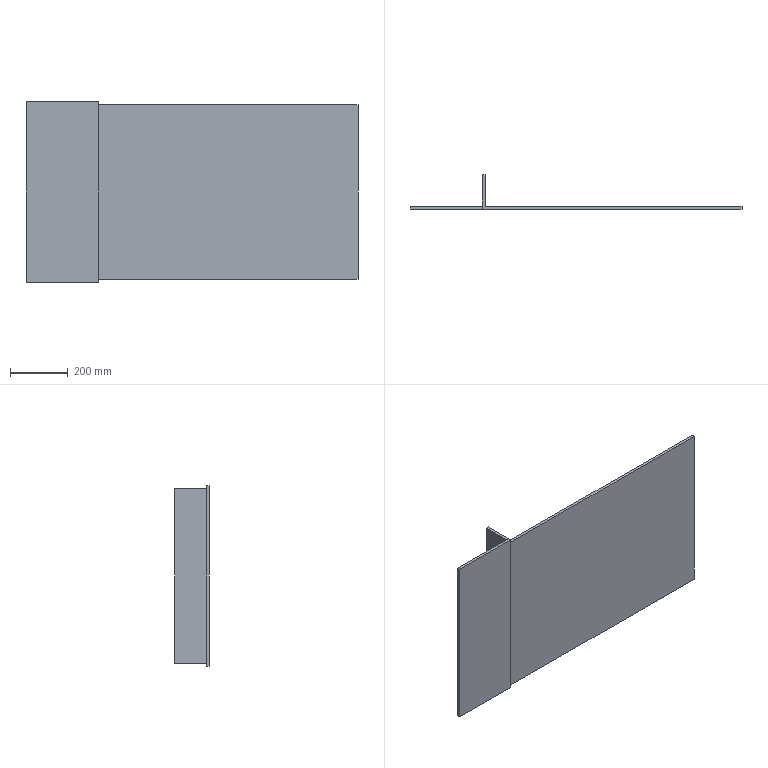Part | STEP file | zhihediban | 2 solids | 14 faces | box 1150 x 120 x 626 mm | volume 7685600 mm3 | plane 14
STEP:
#1=CARTESIAN_POINT('',(0.,0.,0.));
#2=DIRECTION('',(0.,0.,1.));
#3=DIRECTION('',(1.,0.,0.));
#4=AXIS2_PLACEMENT_3D('',#1,#2,#3);
#5=CARTESIAN_POINT('',(450.,5.,-303.));
#6=VERTEX_POINT('',#5);
#7=CARTESIAN_POINT('',(-440.,5.,-303.));
#8=VERTEX_POINT('',#7);
#9=CARTESIAN_POINT('',(-450.,5.,-303.));
#10=DIRECTION('',(-1.,0.,0.));
#11=VECTOR('',#10,1.);
#12=LINE('',#9,#11);
#13=CARTESIAN_POINT('',(0.,5.,0.));
#14=DIRECTION('',(0.,1.,0.));
#15=DIRECTION('',(0.,0.,1.));
#16=AXIS2_PLACEMENT_3D('',#13,#14,#15);
#17=PLANE('',#16);
#18=CARTESIAN_POINT('',(-303.,-450.));
#19=DIRECTION('',(0.,-1.));
#20=VECTOR('',#19,1.);
#21=LINE('',#18,#20);
#22=(GEOMETRIC_REPRESENTATION_CONTEXT(2)PARAMETRIC_REPRESENTATION_CONTEXT()REPRESENTATION_CONTEXT('',''));
#23=DEFINITIONAL_REPRESENTATION('',(#21),#22);
#24=PCURVE('',#17,#23);
#25=CARTESIAN_POINT('',(-450.,5.,-303.));
#26=DIRECTION('',(0.,0.,1.));
#27=DIRECTION('',(1.,0.,0.));
#28=AXIS2_PLACEMENT_3D('',#25,#26,#27);
#29=PLANE('',#28);
#30=CARTESIAN_POINT('',(0.,0.));
#31=DIRECTION('',(-1.,0.));
#32=VECTOR('',#31,1.);
#33=LINE('',#30,#32);
#34=(GEOMETRIC_REPRESENTATION_CONTEXT(2)PARAMETRIC_REPRESENTATION_CONTEXT()REPRESENTATION_CONTEXT('',''));
#35=DEFINITIONAL_REPRESENTATION('',(#33),#34);
#36=PCURVE('',#29,#35);
#37=SURFACE_CURVE('',#12,(#24,#36),.PCURVE_S1.);
#38=EDGE_CURVE('',#6,#8,#37,.T.);
#39=ORIENTED_EDGE('',*,*,#38,.T.);
#40=CARTESIAN_POINT('',(-440.,5.,303.));
#41=VERTEX_POINT('',#40);
#42=CARTESIAN_POINT('',(-440.,5.,-303.));
#43=DIRECTION('',(0.,0.,1.));
#44=VECTOR('',#43,1.);
#45=LINE('',#42,#44);
#46=CARTESIAN_POINT('',(-303.,-440.));
#47=DIRECTION('',(1.,0.));
#48=VECTOR('',#47,1.);
#49=LINE('',#46,#48);
#50=(GEOMETRIC_REPRESENTATION_CONTEXT(2)PARAMETRIC_REPRESENTATION_CONTEXT()REPRESENTATION_CONTEXT('',''));
#51=DEFINITIONAL_REPRESENTATION('',(#49),#50);
#52=PCURVE('',#17,#51);
#53=CARTESIAN_POINT('',(-440.,0.,0.));
#54=DIRECTION('',(1.,0.,0.));
#55=DIRECTION('',(0.,0.,-1.));
#56=AXIS2_PLACEMENT_3D('',#53,#54,#55);
#57=PLANE('',#56);
#58=CARTESIAN_POINT('',(303.,5.));
#59=DIRECTION('',(-1.,0.));
#60=VECTOR('',#59,1.);
#61=LINE('',#58,#60);
#62=(GEOMETRIC_REPRESENTATION_CONTEXT(2)PARAMETRIC_REPRESENTATION_CONTEXT()REPRESENTATION_CONTEXT('',''));
#63=DEFINITIONAL_REPRESENTATION('',(#61),#62);
#64=PCURVE('',#57,#63);
#65=SURFACE_CURVE('',#45,(#52,#64),.PCURVE_S1.);
#66=EDGE_CURVE('',#8,#41,#65,.T.);
#67=ORIENTED_EDGE('',*,*,#66,.T.);
#68=CARTESIAN_POINT('',(450.,5.,303.));
#69=VERTEX_POINT('',#68);
#70=CARTESIAN_POINT('',(-450.,5.,303.));
#71=DIRECTION('',(1.,0.,0.));
#72=VECTOR('',#71,1.);
#73=LINE('',#70,#72);
#74=CARTESIAN_POINT('',(303.,-450.));
#75=DIRECTION('',(0.,1.));
#76=VECTOR('',#75,1.);
#77=LINE('',#74,#76);
#78=(GEOMETRIC_REPRESENTATION_CONTEXT(2)PARAMETRIC_REPRESENTATION_CONTEXT()REPRESENTATION_CONTEXT('',''));
#79=DEFINITIONAL_REPRESENTATION('',(#77),#78);
#80=PCURVE('',#17,#79);
#81=CARTESIAN_POINT('',(-450.,5.,303.));
#82=DIRECTION('',(0.,0.,-1.));
#83=DIRECTION('',(-1.,0.,0.));
#84=AXIS2_PLACEMENT_3D('',#81,#82,#83);
#85=PLANE('',#84);
#86=CARTESIAN_POINT('',(0.,0.));
#87=DIRECTION('',(-1.,0.));
#88=VECTOR('',#87,1.);
#89=LINE('',#86,#88);
#90=(GEOMETRIC_REPRESENTATION_CONTEXT(2)PARAMETRIC_REPRESENTATION_CONTEXT()REPRESENTATION_CONTEXT('',''));
#91=DEFINITIONAL_REPRESENTATION('',(#89),#90);
#92=PCURVE('',#85,#91);
#93=SURFACE_CURVE('',#73,(#80,#92),.PCURVE_S1.);
#94=EDGE_CURVE('',#41,#69,#93,.T.);
#95=ORIENTED_EDGE('',*,*,#94,.T.);
#96=CARTESIAN_POINT('',(450.,5.,-303.));
#97=DIRECTION('',(0.,0.,-1.));
#98=VECTOR('',#97,1.);
#99=LINE('',#96,#98);
#100=CARTESIAN_POINT('',(-303.,450.));
#101=DIRECTION('',(-1.,0.));
#102=VECTOR('',#101,1.);
#103=LINE('',#100,#102);
#104=(GEOMETRIC_REPRESENTATION_CONTEXT(2)PARAMETRIC_REPRESENTATION_CONTEXT()REPRESENTATION_CONTEXT('',''));
#105=DEFINITIONAL_REPRESENTATION('',(#103),#104);
#106=PCURVE('',#17,#105);
#107=CARTESIAN_POINT('',(450.,5.,-303.));
#108=DIRECTION('',(-1.,0.,0.));
#109=DIRECTION('',(0.,0.,1.));
#110=AXIS2_PLACEMENT_3D('',#107,#108,#109);
#111=PLANE('',#110);
#112=CARTESIAN_POINT('',(0.,0.));
#113=DIRECTION('',(-1.,0.));
#114=VECTOR('',#113,1.);
#115=LINE('',#112,#114);
#116=(GEOMETRIC_REPRESENTATION_CONTEXT(2)PARAMETRIC_REPRESENTATION_CONTEXT()REPRESENTATION_CONTEXT('',''));
#117=DEFINITIONAL_REPRESENTATION('',(#115),#116);
#118=PCURVE('',#111,#117);
#119=SURFACE_CURVE('',#99,(#106,#118),.PCURVE_S1.);
#120=EDGE_CURVE('',#69,#6,#119,.T.);
#121=ORIENTED_EDGE('',*,*,#120,.T.);
#122=EDGE_LOOP('',(#39,#67,#95,#121));
#123=FACE_BOUND('',#122,.T.);
#124=ADVANCED_FACE('',(#123),#17,.T.);
#125=CARTESIAN_POINT('',(450.,-5.,303.));
#126=VERTEX_POINT('',#125);
#127=CARTESIAN_POINT('',(450.,-5.,-303.));
#128=VERTEX_POINT('',#127);
#129=CARTESIAN_POINT('',(450.,-5.,-303.));
#130=DIRECTION('',(0.,0.,-1.));
#131=VECTOR('',#130,1.);
#132=LINE('',#129,#131);
#133=CARTESIAN_POINT('',(0.,-10.));
#134=DIRECTION('',(-1.,0.));
#135=VECTOR('',#134,1.);
#136=LINE('',#133,#135);
#137=(GEOMETRIC_REPRESENTATION_CONTEXT(2)PARAMETRIC_REPRESENTATION_CONTEXT()REPRESENTATION_CONTEXT('',''));
#138=DEFINITIONAL_REPRESENTATION('',(#136),#137);
#139=PCURVE('',#111,#138);
#140=CARTESIAN_POINT('',(0.,-5.,0.));
#141=DIRECTION('',(0.,1.,0.));
#142=DIRECTION('',(0.,0.,1.));
#143=AXIS2_PLACEMENT_3D('',#140,#141,#142);
#144=PLANE('',#143);
#145=CARTESIAN_POINT('',(-303.,450.));
#146=DIRECTION('',(-1.,0.));
#147=VECTOR('',#146,1.);
#148=LINE('',#145,#147);
#149=(GEOMETRIC_REPRESENTATION_CONTEXT(2)PARAMETRIC_REPRESENTATION_CONTEXT()REPRESENTATION_CONTEXT('',''));
#150=DEFINITIONAL_REPRESENTATION('',(#148),#149);
#151=PCURVE('',#144,#150);
#152=SURFACE_CURVE('',#132,(#139,#151),.PCURVE_S1.);
#153=EDGE_CURVE('',#126,#128,#152,.T.);
#154=ORIENTED_EDGE('',*,*,#153,.T.);
#155=CARTESIAN_POINT('',(450.,5.,-303.));
#156=DIRECTION('',(0.,-1.,0.));
#157=VECTOR('',#156,1.);
#158=LINE('',#155,#157);
#159=CARTESIAN_POINT('',(0.,0.));
#160=DIRECTION('',(0.,-1.));
#161=VECTOR('',#160,1.);
#162=LINE('',#159,#161);
#163=(GEOMETRIC_REPRESENTATION_CONTEXT(2)PARAMETRIC_REPRESENTATION_CONTEXT()REPRESENTATION_CONTEXT('',''));
#164=DEFINITIONAL_REPRESENTATION('',(#162),#163);
#165=PCURVE('',#111,#164);
#166=CARTESIAN_POINT('',(900.,0.));
#167=DIRECTION('',(0.,-1.));
#168=VECTOR('',#167,1.);
#169=LINE('',#166,#168);
#170=(GEOMETRIC_REPRESENTATION_CONTEXT(2)PARAMETRIC_REPRESENTATION_CONTEXT()REPRESENTATION_CONTEXT('',''));
#171=DEFINITIONAL_REPRESENTATION('',(#169),#170);
#172=PCURVE('',#29,#171);
#173=SURFACE_CURVE('',#158,(#165,#172),.PCURVE_S1.);
#174=EDGE_CURVE('',#6,#128,#173,.T.);
#175=ORIENTED_EDGE('',*,*,#174,.F.);
#176=ORIENTED_EDGE('',*,*,#120,.F.);
#177=CARTESIAN_POINT('',(450.,5.,303.));
#178=DIRECTION('',(0.,-1.,0.));
#179=VECTOR('',#178,1.);
#180=LINE('',#177,#179);
#181=CARTESIAN_POINT('',(606.,0.));
#182=DIRECTION('',(0.,-1.));
#183=VECTOR('',#182,1.);
#184=LINE('',#181,#183);
#185=(GEOMETRIC_REPRESENTATION_CONTEXT(2)PARAMETRIC_REPRESENTATION_CONTEXT()REPRESENTATION_CONTEXT('',''));
#186=DEFINITIONAL_REPRESENTATION('',(#184),#185);
#187=PCURVE('',#111,#186);
#188=CARTESIAN_POINT('',(-900.,0.));
#189=DIRECTION('',(0.,-1.));
#190=VECTOR('',#189,1.);
#191=LINE('',#188,#190);
#192=(GEOMETRIC_REPRESENTATION_CONTEXT(2)PARAMETRIC_REPRESENTATION_CONTEXT()REPRESENTATION_CONTEXT('',''));
#193=DEFINITIONAL_REPRESENTATION('',(#191),#192);
#194=PCURVE('',#85,#193);
#195=SURFACE_CURVE('',#180,(#187,#194),.PCURVE_S1.);
#196=EDGE_CURVE('',#69,#126,#195,.T.);
#197=ORIENTED_EDGE('',*,*,#196,.T.);
#198=EDGE_LOOP('',(#154,#175,#176,#197));
#199=FACE_BOUND('',#198,.T.);
#200=ADVANCED_FACE('',(#199),#111,.F.);
#201=CARTESIAN_POINT('',(-450.,-5.,-303.));
#202=VERTEX_POINT('',#201);
#203=CARTESIAN_POINT('',(-450.,-5.,-303.));
#204=DIRECTION('',(-1.,0.,0.));
#205=VECTOR('',#204,1.);
#206=LINE('',#203,#205);
#207=CARTESIAN_POINT('',(0.,-10.));
#208=DIRECTION('',(-1.,0.));
#209=VECTOR('',#208,1.);
#210=LINE('',#207,#209);
#211=(GEOMETRIC_REPRESENTATION_CONTEXT(2)PARAMETRIC_REPRESENTATION_CONTEXT()REPRESENTATION_CONTEXT('',''));
#212=DEFINITIONAL_REPRESENTATION('',(#210),#211);
#213=PCURVE('',#29,#212);
#214=CARTESIAN_POINT('',(-303.,-450.));
#215=DIRECTION('',(0.,-1.));
#216=VECTOR('',#215,1.);
#217=LINE('',#214,#216);
#218=(GEOMETRIC_REPRESENTATION_CONTEXT(2)PARAMETRIC_REPRESENTATION_CONTEXT()REPRESENTATION_CONTEXT('',''));
#219=DEFINITIONAL_REPRESENTATION('',(#217),#218);
#220=PCURVE('',#144,#219);
#221=SURFACE_CURVE('',#206,(#213,#220),.PCURVE_S1.);
#222=EDGE_CURVE('',#128,#202,#221,.T.);
#223=ORIENTED_EDGE('',*,*,#222,.T.);
#224=CARTESIAN_POINT('',(-450.,115.,-303.));
#225=VERTEX_POINT('',#224);
#226=CARTESIAN_POINT('',(-450.,5.,-303.));
#227=DIRECTION('',(0.,-1.,0.));
#228=VECTOR('',#227,1.);
#229=LINE('',#226,#228);
#230=CARTESIAN_POINT('',(0.,0.));
#231=DIRECTION('',(0.,-1.));
#232=VECTOR('',#231,1.);
#233=LINE('',#230,#232);
#234=(GEOMETRIC_REPRESENTATION_CONTEXT(2)PARAMETRIC_REPRESENTATION_CONTEXT()REPRESENTATION_CONTEXT('',''));
#235=DEFINITIONAL_REPRESENTATION('',(#233),#234);
#236=PCURVE('',#29,#235);
#237=CARTESIAN_POINT('',(-450.,5.,-303.));
#238=DIRECTION('',(1.,0.,0.));
#239=DIRECTION('',(0.,0.,-1.));
#240=AXIS2_PLACEMENT_3D('',#237,#238,#239);
#241=PLANE('',#240);
#242=CARTESIAN_POINT('',(0.,0.));
#243=DIRECTION('',(0.,-1.));
#244=VECTOR('',#243,1.);
#245=LINE('',#242,#244);
#246=(GEOMETRIC_REPRESENTATION_CONTEXT(2)PARAMETRIC_REPRESENTATION_CONTEXT()REPRESENTATION_CONTEXT('',''));
#247=DEFINITIONAL_REPRESENTATION('',(#245),#246);
#248=PCURVE('',#241,#247);
#249=SURFACE_CURVE('',#229,(#236,#248),.PCURVE_S1.);
#250=EDGE_CURVE('',#225,#202,#249,.T.);
#251=ORIENTED_EDGE('',*,*,#250,.F.);
#252=CARTESIAN_POINT('',(-440.,115.,-303.));
#253=VERTEX_POINT('',#252);
#254=CARTESIAN_POINT('',(-440.,115.,-303.));
#255=DIRECTION('',(-1.,0.,0.));
#256=VECTOR('',#255,1.);
#257=LINE('',#254,#256);
#258=CARTESIAN_POINT('',(10.,110.));
#259=DIRECTION('',(-1.,0.));
#260=VECTOR('',#259,1.);
#261=LINE('',#258,#260);
#262=(GEOMETRIC_REPRESENTATION_CONTEXT(2)PARAMETRIC_REPRESENTATION_CONTEXT()REPRESENTATION_CONTEXT('',''));
#263=DEFINITIONAL_REPRESENTATION('',(#261),#262);
#264=PCURVE('',#29,#263);
#265=CARTESIAN_POINT('',(-440.,115.,-303.));
#266=DIRECTION('',(0.,1.,0.));
#267=DIRECTION('',(0.,0.,1.));
#268=AXIS2_PLACEMENT_3D('',#265,#266,#267);
#269=PLANE('',#268);
#270=CARTESIAN_POINT('',(0.,0.));
#271=DIRECTION('',(0.,-1.));
#272=VECTOR('',#271,1.);
#273=LINE('',#270,#272);
#274=(GEOMETRIC_REPRESENTATION_CONTEXT(2)PARAMETRIC_REPRESENTATION_CONTEXT()REPRESENTATION_CONTEXT('',''));
#275=DEFINITIONAL_REPRESENTATION('',(#273),#274);
#276=PCURVE('',#269,#275);
#277=SURFACE_CURVE('',#257,(#264,#276),.PCURVE_S1.);
#278=EDGE_CURVE('',#253,#225,#277,.T.);
#279=ORIENTED_EDGE('',*,*,#278,.F.);
#280=CARTESIAN_POINT('',(-440.,5.,-303.));
#281=DIRECTION('',(0.,-1.,0.));
#282=VECTOR('',#281,1.);
#283=LINE('',#280,#282);
#284=CARTESIAN_POINT('',(10.,0.));
#285=DIRECTION('',(0.,-1.));
#286=VECTOR('',#285,1.);
#287=LINE('',#284,#286);
#288=(GEOMETRIC_REPRESENTATION_CONTEXT(2)PARAMETRIC_REPRESENTATION_CONTEXT()REPRESENTATION_CONTEXT('',''));
#289=DEFINITIONAL_REPRESENTATION('',(#287),#288);
#290=PCURVE('',#29,#289);
#291=CARTESIAN_POINT('',(303.,5.));
#292=DIRECTION('',(0.,-1.));
#293=VECTOR('',#292,1.);
#294=LINE('',#291,#293);
#295=(GEOMETRIC_REPRESENTATION_CONTEXT(2)PARAMETRIC_REPRESENTATION_CONTEXT()REPRESENTATION_CONTEXT('',''));
#296=DEFINITIONAL_REPRESENTATION('',(#294),#295);
#297=PCURVE('',#57,#296);
#298=SURFACE_CURVE('',#283,(#290,#297),.PCURVE_S1.);
#299=EDGE_CURVE('',#253,#8,#298,.T.);
#300=ORIENTED_EDGE('',*,*,#299,.T.);
#301=ORIENTED_EDGE('',*,*,#38,.F.);
#302=ORIENTED_EDGE('',*,*,#174,.T.);
#303=EDGE_LOOP('',(#223,#251,#279,#300,#301,#302));
#304=FACE_BOUND('',#303,.T.);
#305=ADVANCED_FACE('',(#304),#29,.F.);
#306=CARTESIAN_POINT('',(-450.,-5.,303.));
#307=VERTEX_POINT('',#306);
#308=CARTESIAN_POINT('',(-450.,-5.,-303.));
#309=DIRECTION('',(0.,0.,1.));
#310=VECTOR('',#309,1.);
#311=LINE('',#308,#310);
#312=CARTESIAN_POINT('',(0.,-10.));
#313=DIRECTION('',(-1.,0.));
#314=VECTOR('',#313,1.);
#315=LINE('',#312,#314);
#316=(GEOMETRIC_REPRESENTATION_CONTEXT(2)PARAMETRIC_REPRESENTATION_CONTEXT()REPRESENTATION_CONTEXT('',''));
#317=DEFINITIONAL_REPRESENTATION('',(#315),#316);
#318=PCURVE('',#241,#317);
#319=CARTESIAN_POINT('',(-303.,-450.));
#320=DIRECTION('',(1.,0.));
#321=VECTOR('',#320,1.);
#322=LINE('',#319,#321);
#323=(GEOMETRIC_REPRESENTATION_CONTEXT(2)PARAMETRIC_REPRESENTATION_CONTEXT()REPRESENTATION_CONTEXT('',''));
#324=DEFINITIONAL_REPRESENTATION('',(#322),#323);
#325=PCURVE('',#144,#324);
#326=SURFACE_CURVE('',#311,(#318,#325),.PCURVE_S1.);
#327=EDGE_CURVE('',#202,#307,#326,.T.);
#328=ORIENTED_EDGE('',*,*,#327,.T.);
#329=CARTESIAN_POINT('',(-450.,115.,303.));
#330=VERTEX_POINT('',#329);
#331=CARTESIAN_POINT('',(-450.,5.,303.));
#332=DIRECTION('',(0.,-1.,0.));
#333=VECTOR('',#332,1.);
#334=LINE('',#331,#333);
#335=CARTESIAN_POINT('',(-606.,0.));
#336=DIRECTION('',(0.,-1.));
#337=VECTOR('',#336,1.);
#338=LINE('',#335,#337);
#339=(GEOMETRIC_REPRESENTATION_CONTEXT(2)PARAMETRIC_REPRESENTATION_CONTEXT()REPRESENTATION_CONTEXT('',''));
#340=DEFINITIONAL_REPRESENTATION('',(#338),#339);
#341=PCURVE('',#241,#340);
#342=CARTESIAN_POINT('',(0.,0.));
#343=DIRECTION('',(0.,-1.));
#344=VECTOR('',#343,1.);
#345=LINE('',#342,#344);
#346=(GEOMETRIC_REPRESENTATION_CONTEXT(2)PARAMETRIC_REPRESENTATION_CONTEXT()REPRESENTATION_CONTEXT('',''));
#347=DEFINITIONAL_REPRESENTATION('',(#345),#346);
#348=PCURVE('',#85,#347);
#349=SURFACE_CURVE('',#334,(#341,#348),.PCURVE_S1.);
#350=EDGE_CURVE('',#330,#307,#349,.T.);
#351=ORIENTED_EDGE('',*,*,#350,.F.);
#352=CARTESIAN_POINT('',(-450.,115.,-303.));
#353=DIRECTION('',(0.,0.,-1.));
#354=VECTOR('',#353,1.);
#355=LINE('',#352,#354);
#356=CARTESIAN_POINT('',(0.,110.));
#357=DIRECTION('',(1.,0.));
#358=VECTOR('',#357,1.);
#359=LINE('',#356,#358);
#360=(GEOMETRIC_REPRESENTATION_CONTEXT(2)PARAMETRIC_REPRESENTATION_CONTEXT()REPRESENTATION_CONTEXT('',''));
#361=DEFINITIONAL_REPRESENTATION('',(#359),#360);
#362=PCURVE('',#241,#361);
#363=CARTESIAN_POINT('',(0.,-10.));
#364=DIRECTION('',(-1.,0.));
#365=VECTOR('',#364,1.);
#366=LINE('',#363,#365);
#367=(GEOMETRIC_REPRESENTATION_CONTEXT(2)PARAMETRIC_REPRESENTATION_CONTEXT()REPRESENTATION_CONTEXT('',''));
#368=DEFINITIONAL_REPRESENTATION('',(#366),#367);
#369=PCURVE('',#269,#368);
#370=SURFACE_CURVE('',#355,(#362,#369),.PCURVE_S1.);
#371=EDGE_CURVE('',#330,#225,#370,.T.);
#372=ORIENTED_EDGE('',*,*,#371,.T.);
#373=ORIENTED_EDGE('',*,*,#250,.T.);
#374=EDGE_LOOP('',(#328,#351,#372,#373));
#375=FACE_BOUND('',#374,.T.);
#376=ADVANCED_FACE('',(#375),#241,.F.);
#377=CARTESIAN_POINT('',(-450.,-5.,303.));
#378=DIRECTION('',(1.,0.,0.));
#379=VECTOR('',#378,1.);
#380=LINE('',#377,#379);
#381=CARTESIAN_POINT('',(0.,-10.));
#382=DIRECTION('',(-1.,0.));
#383=VECTOR('',#382,1.);
#384=LINE('',#381,#383);
#385=(GEOMETRIC_REPRESENTATION_CONTEXT(2)PARAMETRIC_REPRESENTATION_CONTEXT()REPRESENTATION_CONTEXT('',''));
#386=DEFINITIONAL_REPRESENTATION('',(#384),#385);
#387=PCURVE('',#85,#386);
#388=CARTESIAN_POINT('',(303.,-450.));
#389=DIRECTION('',(0.,1.));
#390=VECTOR('',#389,1.);
#391=LINE('',#388,#390);
#392=(GEOMETRIC_REPRESENTATION_CONTEXT(2)PARAMETRIC_REPRESENTATION_CONTEXT()REPRESENTATION_CONTEXT('',''));
#393=DEFINITIONAL_REPRESENTATION('',(#391),#392);
#394=PCURVE('',#144,#393);
#395=SURFACE_CURVE('',#380,(#387,#394),.PCURVE_S1.);
#396=EDGE_CURVE('',#307,#126,#395,.T.);
#397=ORIENTED_EDGE('',*,*,#396,.T.);
#398=ORIENTED_EDGE('',*,*,#196,.F.);
#399=ORIENTED_EDGE('',*,*,#94,.F.);
#400=CARTESIAN_POINT('',(-440.,115.,303.));
#401=VERTEX_POINT('',#400);
#402=CARTESIAN_POINT('',(-440.,5.,303.));
#403=DIRECTION('',(0.,1.,0.));
#404=VECTOR('',#403,1.);
#405=LINE('',#402,#404);
#406=CARTESIAN_POINT('',(-10.,0.));
#407=DIRECTION('',(0.,1.));
#408=VECTOR('',#407,1.);
#409=LINE('',#406,#408);
#410=(GEOMETRIC_REPRESENTATION_CONTEXT(2)PARAMETRIC_REPRESENTATION_CONTEXT()REPRESENTATION_CONTEXT('',''));
#411=DEFINITIONAL_REPRESENTATION('',(#409),#410);
#412=PCURVE('',#85,#411);
#413=CARTESIAN_POINT('',(-303.,5.));
#414=DIRECTION('',(0.,1.));
#415=VECTOR('',#414,1.);
#416=LINE('',#413,#415);
#417=(GEOMETRIC_REPRESENTATION_CONTEXT(2)PARAMETRIC_REPRESENTATION_CONTEXT()REPRESENTATION_CONTEXT('',''));
#418=DEFINITIONAL_REPRESENTATION('',(#416),#417);
#419=PCURVE('',#57,#418);
#420=SURFACE_CURVE('',#405,(#412,#419),.PCURVE_S1.);
#421=EDGE_CURVE('',#41,#401,#420,.T.);
#422=ORIENTED_EDGE('',*,*,#421,.T.);
#423=CARTESIAN_POINT('',(-440.,115.,303.));
#424=DIRECTION('',(-1.,0.,0.));
#425=VECTOR('',#424,1.);
#426=LINE('',#423,#425);
#427=CARTESIAN_POINT('',(-10.,110.));
#428=DIRECTION('',(1.,0.));
#429=VECTOR('',#428,1.);
#430=LINE('',#427,#429);
#431=(GEOMETRIC_REPRESENTATION_CONTEXT(2)PARAMETRIC_REPRESENTATION_CONTEXT()REPRESENTATION_CONTEXT('',''));
#432=DEFINITIONAL_REPRESENTATION('',(#430),#431);
#433=PCURVE('',#85,#432);
#434=CARTESIAN_POINT('',(606.,0.));
#435=DIRECTION('',(0.,-1.));
#436=VECTOR('',#435,1.);
#437=LINE('',#434,#436);
#438=(GEOMETRIC_REPRESENTATION_CONTEXT(2)PARAMETRIC_REPRESENTATION_CONTEXT()REPRESENTATION_CONTEXT('',''));
#439=DEFINITIONAL_REPRESENTATION('',(#437),#438);
#440=PCURVE('',#269,#439);
#441=SURFACE_CURVE('',#426,(#433,#440),.PCURVE_S1.);
#442=EDGE_CURVE('',#401,#330,#441,.T.);
#443=ORIENTED_EDGE('',*,*,#442,.T.);
#444=ORIENTED_EDGE('',*,*,#350,.T.);
#445=EDGE_LOOP('',(#397,#398,#399,#422,#443,#444));
#446=FACE_BOUND('',#445,.T.);
#447=ADVANCED_FACE('',(#446),#85,.F.);
#448=ORIENTED_EDGE('',*,*,#153,.F.);
#449=ORIENTED_EDGE('',*,*,#396,.F.);
#450=ORIENTED_EDGE('',*,*,#327,.F.);
#451=ORIENTED_EDGE('',*,*,#222,.F.);
#452=EDGE_LOOP('',(#448,#449,#450,#451));
#453=FACE_BOUND('',#452,.T.);
#454=ADVANCED_FACE('',(#453),#144,.F.);
#455=ORIENTED_EDGE('',*,*,#371,.F.);
#456=ORIENTED_EDGE('',*,*,#442,.F.);
#457=CARTESIAN_POINT('',(-440.,115.,-303.));
#458=DIRECTION('',(0.,0.,-1.));
#459=VECTOR('',#458,1.);
#460=LINE('',#457,#459);
#461=CARTESIAN_POINT('',(0.,0.));
#462=DIRECTION('',(-1.,0.));
#463=VECTOR('',#462,1.);
#464=LINE('',#461,#463);
#465=(GEOMETRIC_REPRESENTATION_CONTEXT(2)PARAMETRIC_REPRESENTATION_CONTEXT()REPRESENTATION_CONTEXT('',''));
#466=DEFINITIONAL_REPRESENTATION('',(#464),#465);
#467=PCURVE('',#269,#466);
#468=CARTESIAN_POINT('',(303.,115.));
#469=DIRECTION('',(1.,0.));
#470=VECTOR('',#469,1.);
#471=LINE('',#468,#470);
#472=(GEOMETRIC_REPRESENTATION_CONTEXT(2)PARAMETRIC_REPRESENTATION_CONTEXT()REPRESENTATION_CONTEXT('',''));
#473=DEFINITIONAL_REPRESENTATION('',(#471),#472);
#474=PCURVE('',#57,#473);
#475=SURFACE_CURVE('',#460,(#467,#474),.PCURVE_S1.);
#476=EDGE_CURVE('',#401,#253,#475,.T.);
#477=ORIENTED_EDGE('',*,*,#476,.T.);
#478=ORIENTED_EDGE('',*,*,#278,.T.);
#479=EDGE_LOOP('',(#455,#456,#477,#478));
#480=FACE_BOUND('',#479,.T.);
#481=ADVANCED_FACE('',(#480),#269,.T.);
#482=ORIENTED_EDGE('',*,*,#299,.F.);
#483=ORIENTED_EDGE('',*,*,#476,.F.);
#484=ORIENTED_EDGE('',*,*,#421,.F.);
#485=ORIENTED_EDGE('',*,*,#66,.F.);
#486=EDGE_LOOP('',(#482,#483,#484,#485));
#487=FACE_BOUND('',#486,.T.);
#488=ADVANCED_FACE('',(#487),#57,.T.);
#489=CLOSED_SHELL('',(#124,#200,#305,#376,#447,#454,#481,#488));
#490=MANIFOLD_SOLID_BREP('',#489);
#491=CARTESIAN_POINT('',(-700.,5.,313.));
#492=VERTEX_POINT('',#491);
#493=CARTESIAN_POINT('',(-700.,5.,-313.));
#494=VERTEX_POINT('',#493);
#495=CARTESIAN_POINT('',(-700.,5.,313.));
#496=DIRECTION('',(0.,0.,-1.));
#497=VECTOR('',#496,1.);
#498=LINE('',#495,#497);
#499=CARTESIAN_POINT('',(-700.,5.,313.));
#500=DIRECTION('',(1.,0.,0.));
#501=DIRECTION('',(0.,0.,-1.));
#502=AXIS2_PLACEMENT_3D('',#499,#500,#501);
#503=PLANE('',#502);
#504=CARTESIAN_POINT('',(0.,0.));
#505=DIRECTION('',(1.,0.));
#506=VECTOR('',#505,1.);
#507=LINE('',#504,#506);
#508=(GEOMETRIC_REPRESENTATION_CONTEXT(2)PARAMETRIC_REPRESENTATION_CONTEXT()REPRESENTATION_CONTEXT('',''));
#509=DEFINITIONAL_REPRESENTATION('',(#507),#508);
#510=PCURVE('',#503,#509);
#511=CARTESIAN_POINT('',(-700.,5.,313.));
#512=DIRECTION('',(0.,-1.,0.));
#513=DIRECTION('',(0.,0.,-1.));
#514=AXIS2_PLACEMENT_3D('',#511,#512,#513);
#515=PLANE('',#514);
#516=CARTESIAN_POINT('',(0.,0.));
#517=DIRECTION('',(1.,0.));
#518=VECTOR('',#517,1.);
#519=LINE('',#516,#518);
#520=(GEOMETRIC_REPRESENTATION_CONTEXT(2)PARAMETRIC_REPRESENTATION_CONTEXT()REPRESENTATION_CONTEXT('',''));
#521=DEFINITIONAL_REPRESENTATION('',(#519),#520);
#522=PCURVE('',#515,#521);
#523=SURFACE_CURVE('',#498,(#510,#522),.PCURVE_S1.);
#524=EDGE_CURVE('',#492,#494,#523,.T.);
#525=ORIENTED_EDGE('',*,*,#524,.T.);
#526=CARTESIAN_POINT('',(-700.,-5.,-313.));
#527=VERTEX_POINT('',#526);
#528=CARTESIAN_POINT('',(-700.,5.,-313.));
#529=DIRECTION('',(0.,-1.,0.));
#530=VECTOR('',#529,1.);
#531=LINE('',#528,#530);
#532=CARTESIAN_POINT('',(626.,0.));
#533=DIRECTION('',(0.,-1.));
#534=VECTOR('',#533,1.);
#535=LINE('',#532,#534);
#536=(GEOMETRIC_REPRESENTATION_CONTEXT(2)PARAMETRIC_REPRESENTATION_CONTEXT()REPRESENTATION_CONTEXT('',''));
#537=DEFINITIONAL_REPRESENTATION('',(#535),#536);
#538=PCURVE('',#503,#537);
#539=CARTESIAN_POINT('',(0.,0.,-313.));
#540=DIRECTION('',(0.,0.,1.));
#541=DIRECTION('',(1.,0.,0.));
#542=AXIS2_PLACEMENT_3D('',#539,#540,#541);
#543=PLANE('',#542);
#544=CARTESIAN_POINT('',(-700.,5.));
#545=DIRECTION('',(0.,-1.));
#546=VECTOR('',#545,1.);
#547=LINE('',#544,#546);
#548=(GEOMETRIC_REPRESENTATION_CONTEXT(2)PARAMETRIC_REPRESENTATION_CONTEXT()REPRESENTATION_CONTEXT('',''));
#549=DEFINITIONAL_REPRESENTATION('',(#547),#548);
#550=PCURVE('',#543,#549);
#551=SURFACE_CURVE('',#531,(#538,#550),.PCURVE_S1.);
#552=EDGE_CURVE('',#494,#527,#551,.T.);
#553=ORIENTED_EDGE('',*,*,#552,.T.);
#554=CARTESIAN_POINT('',(-700.,-5.,313.));
#555=VERTEX_POINT('',#554);
#556=CARTESIAN_POINT('',(-700.,-5.,313.));
#557=DIRECTION('',(0.,0.,-1.));
#558=VECTOR('',#557,1.);
#559=LINE('',#556,#558);
#560=CARTESIAN_POINT('',(0.,-10.));
#561=DIRECTION('',(1.,0.));
#562=VECTOR('',#561,1.);
#563=LINE('',#560,#562);
#564=(GEOMETRIC_REPRESENTATION_CONTEXT(2)PARAMETRIC_REPRESENTATION_CONTEXT()REPRESENTATION_CONTEXT('',''));
#565=DEFINITIONAL_REPRESENTATION('',(#563),#564);
#566=PCURVE('',#503,#565);
#567=CARTESIAN_POINT('',(-700.,-5.,313.));
#568=DIRECTION('',(0.,1.,0.));
#569=DIRECTION('',(0.,0.,1.));
#570=AXIS2_PLACEMENT_3D('',#567,#568,#569);
#571=PLANE('',#570);
#572=CARTESIAN_POINT('',(0.,0.));
#573=DIRECTION('',(-1.,0.));
#574=VECTOR('',#573,1.);
#575=LINE('',#572,#574);
#576=(GEOMETRIC_REPRESENTATION_CONTEXT(2)PARAMETRIC_REPRESENTATION_CONTEXT()REPRESENTATION_CONTEXT('',''));
#577=DEFINITIONAL_REPRESENTATION('',(#575),#576);
#578=PCURVE('',#571,#577);
#579=SURFACE_CURVE('',#559,(#566,#578),.PCURVE_S1.);
#580=EDGE_CURVE('',#555,#527,#579,.T.);
#581=ORIENTED_EDGE('',*,*,#580,.F.);
#582=CARTESIAN_POINT('',(-700.,5.,313.));
#583=DIRECTION('',(0.,-1.,0.));
#584=VECTOR('',#583,1.);
#585=LINE('',#582,#584);
#586=CARTESIAN_POINT('',(0.,0.));
#587=DIRECTION('',(0.,-1.));
#588=VECTOR('',#587,1.);
#589=LINE('',#586,#588);
#590=(GEOMETRIC_REPRESENTATION_CONTEXT(2)PARAMETRIC_REPRESENTATION_CONTEXT()REPRESENTATION_CONTEXT('',''));
#591=DEFINITIONAL_REPRESENTATION('',(#589),#590);
#592=PCURVE('',#503,#591);
#593=CARTESIAN_POINT('',(0.,0.,313.));
#594=DIRECTION('',(0.,0.,1.));
#595=DIRECTION('',(1.,0.,0.));
#596=AXIS2_PLACEMENT_3D('',#593,#594,#595);
#597=PLANE('',#596);
#598=CARTESIAN_POINT('',(-700.,5.));
#599=DIRECTION('',(0.,-1.));
#600=VECTOR('',#599,1.);
#601=LINE('',#598,#600);
#602=(GEOMETRIC_REPRESENTATION_CONTEXT(2)PARAMETRIC_REPRESENTATION_CONTEXT()REPRESENTATION_CONTEXT('',''));
#603=DEFINITIONAL_REPRESENTATION('',(#601),#602);
#604=PCURVE('',#597,#603);
#605=SURFACE_CURVE('',#585,(#592,#604),.PCURVE_S1.);
#606=EDGE_CURVE('',#492,#555,#605,.T.);
#607=ORIENTED_EDGE('',*,*,#606,.F.);
#608=EDGE_LOOP('',(#525,#553,#581,#607));
#609=FACE_BOUND('',#608,.T.);
#610=ADVANCED_FACE('',(#609),#503,.F.);
#611=ORIENTED_EDGE('',*,*,#580,.T.);
#612=CARTESIAN_POINT('',(-450.,-5.,-313.));
#613=VERTEX_POINT('',#612);
#614=CARTESIAN_POINT('',(-700.,-5.,-313.));
#615=DIRECTION('',(1.,0.,0.));
#616=VECTOR('',#615,1.);
#617=LINE('',#614,#616);
#618=CARTESIAN_POINT('',(-626.,0.));
#619=DIRECTION('',(0.,1.));
#620=VECTOR('',#619,1.);
#621=LINE('',#618,#620);
#622=(GEOMETRIC_REPRESENTATION_CONTEXT(2)PARAMETRIC_REPRESENTATION_CONTEXT()REPRESENTATION_CONTEXT('',''));
#623=DEFINITIONAL_REPRESENTATION('',(#621),#622);
#624=PCURVE('',#571,#623);
#625=CARTESIAN_POINT('',(-700.,-5.));
#626=DIRECTION('',(1.,0.));
#627=VECTOR('',#626,1.);
#628=LINE('',#625,#627);
#629=(GEOMETRIC_REPRESENTATION_CONTEXT(2)PARAMETRIC_REPRESENTATION_CONTEXT()REPRESENTATION_CONTEXT('',''));
#630=DEFINITIONAL_REPRESENTATION('',(#628),#629);
#631=PCURVE('',#543,#630);
#632=SURFACE_CURVE('',#617,(#624,#631),.PCURVE_S1.);
#633=EDGE_CURVE('',#527,#613,#632,.T.);
#634=ORIENTED_EDGE('',*,*,#633,.T.);
#635=CARTESIAN_POINT('',(-450.,-5.,313.));
#636=VERTEX_POINT('',#635);
#637=CARTESIAN_POINT('',(-450.,-5.,313.));
#638=DIRECTION('',(0.,0.,-1.));
#639=VECTOR('',#638,1.);
#640=LINE('',#637,#639);
#641=CARTESIAN_POINT('',(0.,250.));
#642=DIRECTION('',(-1.,0.));
#643=VECTOR('',#642,1.);
#644=LINE('',#641,#643);
#645=(GEOMETRIC_REPRESENTATION_CONTEXT(2)PARAMETRIC_REPRESENTATION_CONTEXT()REPRESENTATION_CONTEXT('',''));
#646=DEFINITIONAL_REPRESENTATION('',(#644),#645);
#647=PCURVE('',#571,#646);
#648=CARTESIAN_POINT('',(-450.,5.,313.));
#649=DIRECTION('',(-1.,0.,0.));
#650=DIRECTION('',(0.,0.,1.));
#651=AXIS2_PLACEMENT_3D('',#648,#649,#650);
#652=PLANE('',#651);
#653=CARTESIAN_POINT('',(0.,-10.));
#654=DIRECTION('',(-1.,0.));
#655=VECTOR('',#654,1.);
#656=LINE('',#653,#655);
#657=(GEOMETRIC_REPRESENTATION_CONTEXT(2)PARAMETRIC_REPRESENTATION_CONTEXT()REPRESENTATION_CONTEXT('',''));
#658=DEFINITIONAL_REPRESENTATION('',(#656),#657);
#659=PCURVE('',#652,#658);
#660=SURFACE_CURVE('',#640,(#647,#659),.PCURVE_S1.);
#661=EDGE_CURVE('',#636,#613,#660,.T.);
#662=ORIENTED_EDGE('',*,*,#661,.F.);
#663=CARTESIAN_POINT('',(-700.,-5.,313.));
#664=DIRECTION('',(1.,0.,0.));
#665=VECTOR('',#664,1.);
#666=LINE('',#663,#665);
#667=CARTESIAN_POINT('',(0.,0.));
#668=DIRECTION('',(0.,1.));
#669=VECTOR('',#668,1.);
#670=LINE('',#667,#669);
#671=(GEOMETRIC_REPRESENTATION_CONTEXT(2)PARAMETRIC_REPRESENTATION_CONTEXT()REPRESENTATION_CONTEXT('',''));
#672=DEFINITIONAL_REPRESENTATION('',(#670),#671);
#673=PCURVE('',#571,#672);
#674=CARTESIAN_POINT('',(-700.,-5.));
#675=DIRECTION('',(1.,0.));
#676=VECTOR('',#675,1.);
#677=LINE('',#674,#676);
#678=(GEOMETRIC_REPRESENTATION_CONTEXT(2)PARAMETRIC_REPRESENTATION_CONTEXT()REPRESENTATION_CONTEXT('',''));
#679=DEFINITIONAL_REPRESENTATION('',(#677),#678);
#680=PCURVE('',#597,#679);
#681=SURFACE_CURVE('',#666,(#673,#680),.PCURVE_S1.);
#682=EDGE_CURVE('',#555,#636,#681,.T.);
#683=ORIENTED_EDGE('',*,*,#682,.F.);
#684=EDGE_LOOP('',(#611,#634,#662,#683));
#685=FACE_BOUND('',#684,.T.);
#686=ADVANCED_FACE('',(#685),#571,.F.);
#687=ORIENTED_EDGE('',*,*,#661,.T.);
#688=CARTESIAN_POINT('',(-450.,5.,-313.));
#689=VERTEX_POINT('',#688);
#690=CARTESIAN_POINT('',(-450.,5.,-313.));
#691=DIRECTION('',(0.,1.,0.));
#692=VECTOR('',#691,1.);
#693=LINE('',#690,#692);
#694=CARTESIAN_POINT('',(-626.,0.));
#695=DIRECTION('',(0.,1.));
#696=VECTOR('',#695,1.);
#697=LINE('',#694,#696);
#698=(GEOMETRIC_REPRESENTATION_CONTEXT(2)PARAMETRIC_REPRESENTATION_CONTEXT()REPRESENTATION_CONTEXT('',''));
#699=DEFINITIONAL_REPRESENTATION('',(#697),#698);
#700=PCURVE('',#652,#699);
#701=CARTESIAN_POINT('',(-450.,5.));
#702=DIRECTION('',(0.,1.));
#703=VECTOR('',#702,1.);
#704=LINE('',#701,#703);
#705=(GEOMETRIC_REPRESENTATION_CONTEXT(2)PARAMETRIC_REPRESENTATION_CONTEXT()REPRESENTATION_CONTEXT('',''));
#706=DEFINITIONAL_REPRESENTATION('',(#704),#705);
#707=PCURVE('',#543,#706);
#708=SURFACE_CURVE('',#693,(#700,#707),.PCURVE_S1.);
#709=EDGE_CURVE('',#613,#689,#708,.T.);
#710=ORIENTED_EDGE('',*,*,#709,.T.);
#711=CARTESIAN_POINT('',(-450.,5.,313.));
#712=VERTEX_POINT('',#711);
#713=CARTESIAN_POINT('',(-450.,5.,313.));
#714=DIRECTION('',(0.,0.,-1.));
#715=VECTOR('',#714,1.);
#716=LINE('',#713,#715);
#717=CARTESIAN_POINT('',(0.,0.));
#718=DIRECTION('',(-1.,0.));
#719=VECTOR('',#718,1.);
#720=LINE('',#717,#719);
#721=(GEOMETRIC_REPRESENTATION_CONTEXT(2)PARAMETRIC_REPRESENTATION_CONTEXT()REPRESENTATION_CONTEXT('',''));
#722=DEFINITIONAL_REPRESENTATION('',(#720),#721);
#723=PCURVE('',#652,#722);
#724=CARTESIAN_POINT('',(0.,250.));
#725=DIRECTION('',(1.,0.));
#726=VECTOR('',#725,1.);
#727=LINE('',#724,#726);
#728=(GEOMETRIC_REPRESENTATION_CONTEXT(2)PARAMETRIC_REPRESENTATION_CONTEXT()REPRESENTATION_CONTEXT('',''));
#729=DEFINITIONAL_REPRESENTATION('',(#727),#728);
#730=PCURVE('',#515,#729);
#731=SURFACE_CURVE('',#716,(#723,#730),.PCURVE_S1.);
#732=EDGE_CURVE('',#712,#689,#731,.T.);
#733=ORIENTED_EDGE('',*,*,#732,.F.);
#734=CARTESIAN_POINT('',(-450.,5.,313.));
#735=DIRECTION('',(0.,1.,0.));
#736=VECTOR('',#735,1.);
#737=LINE('',#734,#736);
#738=CARTESIAN_POINT('',(0.,0.));
#739=DIRECTION('',(0.,1.));
#740=VECTOR('',#739,1.);
#741=LINE('',#738,#740);
#742=(GEOMETRIC_REPRESENTATION_CONTEXT(2)PARAMETRIC_REPRESENTATION_CONTEXT()REPRESENTATION_CONTEXT('',''));
#743=DEFINITIONAL_REPRESENTATION('',(#741),#742);
#744=PCURVE('',#652,#743);
#745=CARTESIAN_POINT('',(-450.,5.));
#746=DIRECTION('',(0.,1.));
#747=VECTOR('',#746,1.);
#748=LINE('',#745,#747);
#749=(GEOMETRIC_REPRESENTATION_CONTEXT(2)PARAMETRIC_REPRESENTATION_CONTEXT()REPRESENTATION_CONTEXT('',''));
#750=DEFINITIONAL_REPRESENTATION('',(#748),#749);
#751=PCURVE('',#597,#750);
#752=SURFACE_CURVE('',#737,(#744,#751),.PCURVE_S1.);
#753=EDGE_CURVE('',#636,#712,#752,.T.);
#754=ORIENTED_EDGE('',*,*,#753,.F.);
#755=EDGE_LOOP('',(#687,#710,#733,#754));
#756=FACE_BOUND('',#755,.T.);
#757=ADVANCED_FACE('',(#756),#652,.F.);
#758=ORIENTED_EDGE('',*,*,#732,.T.);
#759=CARTESIAN_POINT('',(-700.,5.,-313.));
#760=DIRECTION('',(-1.,0.,0.));
#761=VECTOR('',#760,1.);
#762=LINE('',#759,#761);
#763=CARTESIAN_POINT('',(626.,0.));
#764=DIRECTION('',(0.,-1.));
#765=VECTOR('',#764,1.);
#766=LINE('',#763,#765);
#767=(GEOMETRIC_REPRESENTATION_CONTEXT(2)PARAMETRIC_REPRESENTATION_CONTEXT()REPRESENTATION_CONTEXT('',''));
#768=DEFINITIONAL_REPRESENTATION('',(#766),#767);
#769=PCURVE('',#515,#768);
#770=CARTESIAN_POINT('',(-700.,5.));
#771=DIRECTION('',(-1.,0.));
#772=VECTOR('',#771,1.);
#773=LINE('',#770,#772);
#774=(GEOMETRIC_REPRESENTATION_CONTEXT(2)PARAMETRIC_REPRESENTATION_CONTEXT()REPRESENTATION_CONTEXT('',''));
#775=DEFINITIONAL_REPRESENTATION('',(#773),#774);
#776=PCURVE('',#543,#775);
#777=SURFACE_CURVE('',#762,(#769,#776),.PCURVE_S1.);
#778=EDGE_CURVE('',#689,#494,#777,.T.);
#779=ORIENTED_EDGE('',*,*,#778,.T.);
#780=ORIENTED_EDGE('',*,*,#524,.F.);
#781=CARTESIAN_POINT('',(-700.,5.,313.));
#782=DIRECTION('',(-1.,0.,0.));
#783=VECTOR('',#782,1.);
#784=LINE('',#781,#783);
#785=CARTESIAN_POINT('',(0.,0.));
#786=DIRECTION('',(0.,-1.));
#787=VECTOR('',#786,1.);
#788=LINE('',#785,#787);
#789=(GEOMETRIC_REPRESENTATION_CONTEXT(2)PARAMETRIC_REPRESENTATION_CONTEXT()REPRESENTATION_CONTEXT('',''));
#790=DEFINITIONAL_REPRESENTATION('',(#788),#789);
#791=PCURVE('',#515,#790);
#792=CARTESIAN_POINT('',(-700.,5.));
#793=DIRECTION('',(-1.,0.));
#794=VECTOR('',#793,1.);
#795=LINE('',#792,#794);
#796=(GEOMETRIC_REPRESENTATION_CONTEXT(2)PARAMETRIC_REPRESENTATION_CONTEXT()REPRESENTATION_CONTEXT('',''));
#797=DEFINITIONAL_REPRESENTATION('',(#795),#796);
#798=PCURVE('',#597,#797);
#799=SURFACE_CURVE('',#784,(#791,#798),.PCURVE_S1.);
#800=EDGE_CURVE('',#712,#492,#799,.T.);
#801=ORIENTED_EDGE('',*,*,#800,.F.);
#802=EDGE_LOOP('',(#758,#779,#780,#801));
#803=FACE_BOUND('',#802,.T.);
#804=ADVANCED_FACE('',(#803),#515,.F.);
#805=ORIENTED_EDGE('',*,*,#606,.T.);
#806=ORIENTED_EDGE('',*,*,#682,.T.);
#807=ORIENTED_EDGE('',*,*,#753,.T.);
#808=ORIENTED_EDGE('',*,*,#800,.T.);
#809=EDGE_LOOP('',(#805,#806,#807,#808));
#810=FACE_BOUND('',#809,.T.);
#811=ADVANCED_FACE('',(#810),#597,.T.);
#812=ORIENTED_EDGE('',*,*,#552,.F.);
#813=ORIENTED_EDGE('',*,*,#778,.F.);
#814=ORIENTED_EDGE('',*,*,#709,.F.);
#815=ORIENTED_EDGE('',*,*,#633,.F.);
#816=EDGE_LOOP('',(#812,#813,#814,#815));
#817=FACE_BOUND('',#816,.T.);
#818=ADVANCED_FACE('',(#817),#543,.F.);
#819=CLOSED_SHELL('',(#610,#686,#757,#804,#811,#818));
#820=MANIFOLD_SOLID_BREP('',#819);
#821=(LENGTH_UNIT()NAMED_UNIT(*)SI_UNIT(.MILLI.,.METRE.));
#822=UNCERTAINTY_MEASURE_WITH_UNIT(LENGTH_MEASURE(0.0000001),#821,'','');
#823=(NAMED_UNIT(*)PLANE_ANGLE_UNIT()SI_UNIT($,.RADIAN.));
#824=(NAMED_UNIT(*)SI_UNIT($,.STERADIAN.)SOLID_ANGLE_UNIT());
#825=(GEOMETRIC_REPRESENTATION_CONTEXT(3)GLOBAL_UNCERTAINTY_ASSIGNED_CONTEXT((#822))GLOBAL_UNIT_ASSIGNED_CONTEXT((#821,#823,#824))REPRESENTATION_CONTEXT('',''));
#826=SHAPE_REPRESENTATION('',(#4,#490,#820),#825);